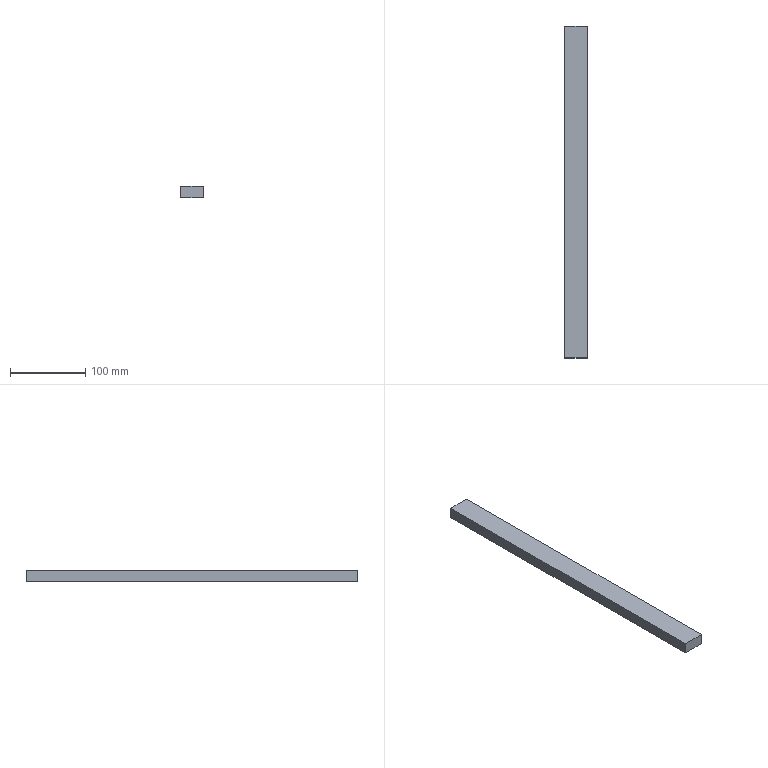Part | NX | features solid 2 | 1 solid | 6 faces | box 30 x 442.5 x 15 mm | volume 199125 mm3 | plane 6
STEP:
#1=CARTESIAN_POINT('',(470.,692.5,-69.));
#2=VERTEX_POINT('',#1);
#3=CARTESIAN_POINT('',(500.,692.5,-69.));
#4=VERTEX_POINT('',#3);
#5=CARTESIAN_POINT('',(620.,692.5,-69.));
#6=DIRECTION('',(1.,0.,0.));
#7=VECTOR('',#6,1000.);
#8=LINE('',#5,#7);
#9=EDGE_CURVE('',#2,#4,#8,.T.);
#10=ORIENTED_EDGE('',*,*,#9,.T.);
#11=CARTESIAN_POINT('',(500.,692.5,-84.));
#12=VERTEX_POINT('',#11);
#13=CARTESIAN_POINT('',(500.,692.5,-84.));
#14=DIRECTION('',(0.,0.,-1.));
#15=VECTOR('',#14,1000.);
#16=LINE('',#13,#15);
#17=EDGE_CURVE('',#12,#4,#16,.F.);
#18=ORIENTED_EDGE('',*,*,#17,.F.);
#19=CARTESIAN_POINT('',(470.,692.5,-84.));
#20=VERTEX_POINT('',#19);
#21=CARTESIAN_POINT('',(620.,692.5,-84.));
#22=DIRECTION('',(-1.,0.,0.));
#23=VECTOR('',#22,1000.);
#24=LINE('',#21,#23);
#25=EDGE_CURVE('',#20,#12,#24,.F.);
#26=ORIENTED_EDGE('',*,*,#25,.F.);
#27=CARTESIAN_POINT('',(470.,692.5,-84.));
#28=DIRECTION('',(0.,0.,-1.));
#29=VECTOR('',#28,1000.);
#30=LINE('',#27,#29);
#31=EDGE_CURVE('',#20,#2,#30,.F.);
#32=ORIENTED_EDGE('',*,*,#31,.T.);
#33=EDGE_LOOP('',(#10,#18,#26,#32));
#34=FACE_BOUND('',#33,.T.);
#35=CARTESIAN_POINT('',(620.,692.5,-84.));
#36=DIRECTION('',(0.,1.,0.));
#37=DIRECTION('',(0.,0.,1.));
#38=AXIS2_PLACEMENT_3D('',#35,#36,#37);
#39=PLANE('',#38);
#40=ADVANCED_FACE('',(#34),#39,.T.);
#41=ORIENTED_EDGE('',*,*,#25,.T.);
#42=CARTESIAN_POINT('',(500.,250.,-84.));
#43=VERTEX_POINT('',#42);
#44=CARTESIAN_POINT('',(500.,672.5,-84.));
#45=DIRECTION('',(0.,-1.,0.));
#46=VECTOR('',#45,1000.);
#47=LINE('',#44,#46);
#48=EDGE_CURVE('',#12,#43,#47,.T.);
#49=ORIENTED_EDGE('',*,*,#48,.T.);
#50=CARTESIAN_POINT('',(470.,250.,-84.));
#51=VERTEX_POINT('',#50);
#52=CARTESIAN_POINT('',(522.5,250.,-84.));
#53=DIRECTION('',(-1.,0.,0.));
#54=VECTOR('',#53,1000.);
#55=LINE('',#52,#54);
#56=EDGE_CURVE('',#51,#43,#55,.F.);
#57=ORIENTED_EDGE('',*,*,#56,.F.);
#58=CARTESIAN_POINT('',(470.,672.5,-84.));
#59=DIRECTION('',(0.,-1.,0.));
#60=VECTOR('',#59,1000.);
#61=LINE('',#58,#60);
#62=EDGE_CURVE('',#20,#51,#61,.T.);
#63=ORIENTED_EDGE('',*,*,#62,.F.);
#64=EDGE_LOOP('',(#41,#49,#57,#63));
#65=FACE_BOUND('',#64,.T.);
#66=CARTESIAN_POINT('',(620.,672.5,-84.));
#67=DIRECTION('',(0.,0.,1.));
#68=DIRECTION('',(0.,-1.,0.));
#69=AXIS2_PLACEMENT_3D('',#66,#67,#68);
#70=PLANE('',#69);
#71=ADVANCED_FACE('',(#65),#70,.F.);
#72=ORIENTED_EDGE('',*,*,#56,.T.);
#73=CARTESIAN_POINT('',(500.,250.,-69.));
#74=VERTEX_POINT('',#73);
#75=CARTESIAN_POINT('',(500.,250.,-84.));
#76=DIRECTION('',(0.,0.,-1.));
#77=VECTOR('',#76,1000.);
#78=LINE('',#75,#77);
#79=EDGE_CURVE('',#43,#74,#78,.F.);
#80=ORIENTED_EDGE('',*,*,#79,.T.);
#81=CARTESIAN_POINT('',(470.,250.,-69.));
#82=VERTEX_POINT('',#81);
#83=CARTESIAN_POINT('',(620.,250.,-69.));
#84=DIRECTION('',(1.,0.,0.));
#85=VECTOR('',#84,1000.);
#86=LINE('',#83,#85);
#87=EDGE_CURVE('',#82,#74,#86,.T.);
#88=ORIENTED_EDGE('',*,*,#87,.F.);
#89=CARTESIAN_POINT('',(470.,250.,-84.));
#90=DIRECTION('',(0.,0.,-1.));
#91=VECTOR('',#90,1000.);
#92=LINE('',#89,#91);
#93=EDGE_CURVE('',#51,#82,#92,.F.);
#94=ORIENTED_EDGE('',*,*,#93,.F.);
#95=EDGE_LOOP('',(#72,#80,#88,#94));
#96=FACE_BOUND('',#95,.T.);
#97=CARTESIAN_POINT('',(522.5,250.,-69.));
#98=DIRECTION('',(0.,-1.,0.));
#99=DIRECTION('',(-1.,0.,0.));
#100=AXIS2_PLACEMENT_3D('',#97,#98,#99);
#101=PLANE('',#100);
#102=ADVANCED_FACE('',(#96),#101,.T.);
#103=CARTESIAN_POINT('',(470.,672.5,-69.));
#104=DIRECTION('',(0.,1.,0.));
#105=VECTOR('',#104,1000.);
#106=LINE('',#103,#105);
#107=EDGE_CURVE('',#2,#82,#106,.F.);
#108=ORIENTED_EDGE('',*,*,#107,.T.);
#109=ORIENTED_EDGE('',*,*,#87,.T.);
#110=CARTESIAN_POINT('',(500.,672.5,-69.));
#111=DIRECTION('',(0.,1.,0.));
#112=VECTOR('',#111,1000.);
#113=LINE('',#110,#112);
#114=EDGE_CURVE('',#4,#74,#113,.F.);
#115=ORIENTED_EDGE('',*,*,#114,.F.);
#116=ORIENTED_EDGE('',*,*,#9,.F.);
#117=EDGE_LOOP('',(#108,#109,#115,#116));
#118=FACE_BOUND('',#117,.T.);
#119=CARTESIAN_POINT('',(620.,672.5,-69.));
#120=DIRECTION('',(0.,0.,1.));
#121=DIRECTION('',(0.,-1.,0.));
#122=AXIS2_PLACEMENT_3D('',#119,#120,#121);
#123=PLANE('',#122);
#124=ADVANCED_FACE('',(#118),#123,.T.);
#125=ORIENTED_EDGE('',*,*,#79,.F.);
#126=ORIENTED_EDGE('',*,*,#48,.F.);
#127=ORIENTED_EDGE('',*,*,#17,.T.);
#128=ORIENTED_EDGE('',*,*,#114,.T.);
#129=EDGE_LOOP('',(#125,#126,#127,#128));
#130=FACE_BOUND('',#129,.T.);
#131=CARTESIAN_POINT('',(500.,672.5,-84.));
#132=DIRECTION('',(1.,0.,0.));
#133=DIRECTION('',(0.,0.,-1.));
#134=AXIS2_PLACEMENT_3D('',#131,#132,#133);
#135=PLANE('',#134);
#136=ADVANCED_FACE('',(#130),#135,.T.);
#137=ORIENTED_EDGE('',*,*,#93,.T.);
#138=ORIENTED_EDGE('',*,*,#107,.F.);
#139=ORIENTED_EDGE('',*,*,#31,.F.);
#140=ORIENTED_EDGE('',*,*,#62,.T.);
#141=EDGE_LOOP('',(#137,#138,#139,#140));
#142=FACE_BOUND('',#141,.T.);
#143=CARTESIAN_POINT('',(470.,672.5,-84.));
#144=DIRECTION('',(1.,0.,0.));
#145=DIRECTION('',(0.,0.,-1.));
#146=AXIS2_PLACEMENT_3D('',#143,#144,#145);
#147=PLANE('',#146);
#148=ADVANCED_FACE('',(#142),#147,.F.);
#149=CLOSED_SHELL('',(#40,#71,#102,#124,#136,#148));
#150=MANIFOLD_SOLID_BREP('',#149);
#151=(LENGTH_UNIT()NAMED_UNIT(*)SI_UNIT(.MILLI.,.METRE.));
#152=UNCERTAINTY_MEASURE_WITH_UNIT(LENGTH_MEASURE(0.00001),#151,'','');
#153=(NAMED_UNIT(*)PLANE_ANGLE_UNIT()SI_UNIT($,.RADIAN.));
#154=(NAMED_UNIT(*)SI_UNIT($,.STERADIAN.)SOLID_ANGLE_UNIT());
#155=(GEOMETRIC_REPRESENTATION_CONTEXT(3)GLOBAL_UNCERTAINTY_ASSIGNED_CONTEXT((#152))GLOBAL_UNIT_ASSIGNED_CONTEXT((#151,#153,#154))REPRESENTATION_CONTEXT('',''));
#156=ADVANCED_BREP_SHAPE_REPRESENTATION('',(#150),#155);